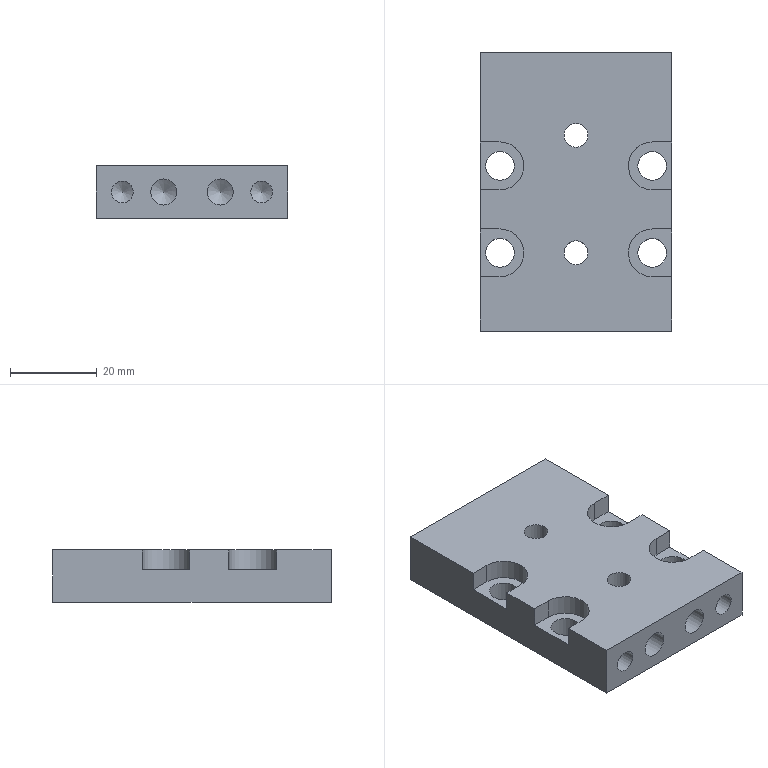Part | NX | features BREP 1 | 1 solid | 40 faces | box 44 x 64 x 12 mm | volume 28668 mm3 | plane 20 | cylinder 16 | cone 4 | commonest cylinder face diameters 6.6 x4 11 x4 5 x2 5.5 x2 6 x2 10 x2
STEP:
#1=CARTESIAN_POINT('',(-22.,-32.,0.));
#2=VERTEX_POINT('',#1);
#3=CARTESIAN_POINT('',(22.,-32.,0.));
#4=VERTEX_POINT('',#3);
#5=CARTESIAN_POINT('',(0.,-32.,0.));
#6=DIRECTION('',(1.,0.,0.));
#7=VECTOR('',#6,1000.);
#8=LINE('',#5,#7);
#9=EDGE_CURVE('',#2,#4,#8,.T.);
#10=ORIENTED_EDGE('',*,*,#9,.F.);
#11=CARTESIAN_POINT('',(-22.,32.,0.));
#12=VERTEX_POINT('',#11);
#13=CARTESIAN_POINT('',(-22.,0.,0.));
#14=DIRECTION('',(0.,-1.,0.));
#15=VECTOR('',#14,1000.);
#16=LINE('',#13,#15);
#17=EDGE_CURVE('',#12,#2,#16,.T.);
#18=ORIENTED_EDGE('',*,*,#17,.F.);
#19=CARTESIAN_POINT('',(22.,32.,0.));
#20=VERTEX_POINT('',#19);
#21=CARTESIAN_POINT('',(0.,32.,0.));
#22=DIRECTION('',(-1.,0.,0.));
#23=VECTOR('',#22,1000.);
#24=LINE('',#21,#23);
#25=EDGE_CURVE('',#20,#12,#24,.T.);
#26=ORIENTED_EDGE('',*,*,#25,.F.);
#27=CARTESIAN_POINT('',(22.,0.,0.));
#28=DIRECTION('',(0.,1.,0.));
#29=VECTOR('',#28,1000.);
#30=LINE('',#27,#29);
#31=EDGE_CURVE('',#4,#20,#30,.T.);
#32=ORIENTED_EDGE('',*,*,#31,.F.);
#33=EDGE_LOOP('',(#10,#18,#26,#32));
#34=FACE_BOUND('',#33,.T.);
#35=CARTESIAN_POINT('',(20.825,-14.,0.));
#36=VERTEX_POINT('',#35);
#37=CARTESIAN_POINT('',(17.525,-14.,0.));
#38=DIRECTION('',(0.,0.,-1.));
#39=DIRECTION('',(1.,0.,0.));
#40=AXIS2_PLACEMENT_3D('',#37,#38,#39);
#41=CIRCLE('',#40,3.3);
#42=EDGE_CURVE('',#36,#36,#41,.T.);
#43=ORIENTED_EDGE('',*,*,#42,.F.);
#44=EDGE_LOOP('',(#43));
#45=FACE_BOUND('',#44,.T.);
#46=CARTESIAN_POINT('',(20.825,6.,0.));
#47=VERTEX_POINT('',#46);
#48=CARTESIAN_POINT('',(17.525,6.,0.));
#49=DIRECTION('',(0.,0.,-1.));
#50=DIRECTION('',(1.,0.,0.));
#51=AXIS2_PLACEMENT_3D('',#48,#49,#50);
#52=CIRCLE('',#51,3.3);
#53=EDGE_CURVE('',#47,#47,#52,.T.);
#54=ORIENTED_EDGE('',*,*,#53,.F.);
#55=EDGE_LOOP('',(#54));
#56=FACE_BOUND('',#55,.T.);
#57=CARTESIAN_POINT('',(-14.175,-14.,0.));
#58=VERTEX_POINT('',#57);
#59=CARTESIAN_POINT('',(-17.475,-14.,0.));
#60=DIRECTION('',(0.,0.,-1.));
#61=DIRECTION('',(1.,0.,0.));
#62=AXIS2_PLACEMENT_3D('',#59,#60,#61);
#63=CIRCLE('',#62,3.3);
#64=EDGE_CURVE('',#58,#58,#63,.T.);
#65=ORIENTED_EDGE('',*,*,#64,.F.);
#66=EDGE_LOOP('',(#65));
#67=FACE_BOUND('',#66,.T.);
#68=CARTESIAN_POINT('',(-14.175,6.,0.));
#69=VERTEX_POINT('',#68);
#70=CARTESIAN_POINT('',(-17.475,6.,0.));
#71=DIRECTION('',(0.,0.,-1.));
#72=DIRECTION('',(1.,0.,0.));
#73=AXIS2_PLACEMENT_3D('',#70,#71,#72);
#74=CIRCLE('',#73,3.3);
#75=EDGE_CURVE('',#69,#69,#74,.T.);
#76=ORIENTED_EDGE('',*,*,#75,.F.);
#77=EDGE_LOOP('',(#76));
#78=FACE_BOUND('',#77,.T.);
#79=CARTESIAN_POINT('',(-5.,-14.,0.));
#80=VERTEX_POINT('',#79);
#81=CARTESIAN_POINT('',(0.,-14.,0.));
#82=DIRECTION('',(0.,0.,-1.));
#83=DIRECTION('',(-1.,0.,0.));
#84=AXIS2_PLACEMENT_3D('',#81,#82,#83);
#85=CIRCLE('',#84,5.);
#86=EDGE_CURVE('',#80,#80,#85,.T.);
#87=ORIENTED_EDGE('',*,*,#86,.F.);
#88=EDGE_LOOP('',(#87));
#89=FACE_BOUND('',#88,.T.);
#90=CARTESIAN_POINT('',(-5.,13.,0.));
#91=VERTEX_POINT('',#90);
#92=CARTESIAN_POINT('',(0.,13.,0.));
#93=DIRECTION('',(0.,0.,-1.));
#94=DIRECTION('',(-1.,0.,0.));
#95=AXIS2_PLACEMENT_3D('',#92,#93,#94);
#96=CIRCLE('',#95,5.);
#97=EDGE_CURVE('',#91,#91,#96,.T.);
#98=ORIENTED_EDGE('',*,*,#97,.F.);
#99=EDGE_LOOP('',(#98));
#100=FACE_BOUND('',#99,.T.);
#101=CARTESIAN_POINT('',(0.,0.,0.));
#102=DIRECTION('',(0.,0.,1.));
#103=DIRECTION('',(-1.,0.,0.));
#104=AXIS2_PLACEMENT_3D('',#101,#102,#103);
#105=PLANE('',#104);
#106=ADVANCED_FACE('',(#34,#45,#56,#67,#78,#89,#100),#105,.F.);
#107=CARTESIAN_POINT('',(22.,-19.5,12.));
#108=VERTEX_POINT('',#107);
#109=CARTESIAN_POINT('',(22.,-19.5,7.4));
#110=VERTEX_POINT('',#109);
#111=CARTESIAN_POINT('',(22.,-19.5,12.));
#112=DIRECTION('',(0.,0.,-1.));
#113=VECTOR('',#112,1000.);
#114=LINE('',#111,#113);
#115=EDGE_CURVE('',#108,#110,#114,.T.);
#116=ORIENTED_EDGE('',*,*,#115,.F.);
#117=CARTESIAN_POINT('',(22.,-32.,12.));
#118=VERTEX_POINT('',#117);
#119=CARTESIAN_POINT('',(22.,32.,12.));
#120=DIRECTION('',(0.,1.,0.));
#121=VECTOR('',#120,1000.);
#122=LINE('',#119,#121);
#123=EDGE_CURVE('',#118,#108,#122,.T.);
#124=ORIENTED_EDGE('',*,*,#123,.F.);
#125=CARTESIAN_POINT('',(22.,-32.,12.));
#126=DIRECTION('',(0.,0.,1.));
#127=VECTOR('',#126,1000.);
#128=LINE('',#125,#127);
#129=EDGE_CURVE('',#4,#118,#128,.T.);
#130=ORIENTED_EDGE('',*,*,#129,.F.);
#131=ORIENTED_EDGE('',*,*,#31,.T.);
#132=CARTESIAN_POINT('',(22.,32.,12.));
#133=VERTEX_POINT('',#132);
#134=CARTESIAN_POINT('',(22.,32.,12.));
#135=DIRECTION('',(0.,0.,-1.));
#136=VECTOR('',#135,1000.);
#137=LINE('',#134,#136);
#138=EDGE_CURVE('',#133,#20,#137,.T.);
#139=ORIENTED_EDGE('',*,*,#138,.F.);
#140=CARTESIAN_POINT('',(22.,11.5,12.));
#141=VERTEX_POINT('',#140);
#142=CARTESIAN_POINT('',(22.,32.,12.));
#143=DIRECTION('',(0.,1.,0.));
#144=VECTOR('',#143,1000.);
#145=LINE('',#142,#144);
#146=EDGE_CURVE('',#141,#133,#145,.T.);
#147=ORIENTED_EDGE('',*,*,#146,.F.);
#148=CARTESIAN_POINT('',(22.,11.5,7.4));
#149=VERTEX_POINT('',#148);
#150=CARTESIAN_POINT('',(22.,11.5,12.));
#151=DIRECTION('',(0.,0.,1.));
#152=VECTOR('',#151,1000.);
#153=LINE('',#150,#152);
#154=EDGE_CURVE('',#149,#141,#153,.T.);
#155=ORIENTED_EDGE('',*,*,#154,.F.);
#156=CARTESIAN_POINT('',(22.,0.5,7.4));
#157=VERTEX_POINT('',#156);
#158=CARTESIAN_POINT('',(22.,32.,7.4));
#159=DIRECTION('',(0.,1.,0.));
#160=VECTOR('',#159,1000.);
#161=LINE('',#158,#160);
#162=EDGE_CURVE('',#157,#149,#161,.T.);
#163=ORIENTED_EDGE('',*,*,#162,.F.);
#164=CARTESIAN_POINT('',(22.,0.5,12.));
#165=VERTEX_POINT('',#164);
#166=CARTESIAN_POINT('',(22.,0.5,12.));
#167=DIRECTION('',(0.,0.,-1.));
#168=VECTOR('',#167,1000.);
#169=LINE('',#166,#168);
#170=EDGE_CURVE('',#165,#157,#169,.T.);
#171=ORIENTED_EDGE('',*,*,#170,.F.);
#172=CARTESIAN_POINT('',(22.,-8.5,12.));
#173=VERTEX_POINT('',#172);
#174=CARTESIAN_POINT('',(22.,32.,12.));
#175=DIRECTION('',(0.,1.,0.));
#176=VECTOR('',#175,1000.);
#177=LINE('',#174,#176);
#178=EDGE_CURVE('',#173,#165,#177,.T.);
#179=ORIENTED_EDGE('',*,*,#178,.F.);
#180=CARTESIAN_POINT('',(22.,-8.5,7.4));
#181=VERTEX_POINT('',#180);
#182=CARTESIAN_POINT('',(22.,-8.5,12.));
#183=DIRECTION('',(0.,0.,1.));
#184=VECTOR('',#183,1000.);
#185=LINE('',#182,#184);
#186=EDGE_CURVE('',#181,#173,#185,.T.);
#187=ORIENTED_EDGE('',*,*,#186,.F.);
#188=CARTESIAN_POINT('',(22.,32.,7.4));
#189=DIRECTION('',(0.,1.,0.));
#190=VECTOR('',#189,1000.);
#191=LINE('',#188,#190);
#192=EDGE_CURVE('',#110,#181,#191,.T.);
#193=ORIENTED_EDGE('',*,*,#192,.F.);
#194=EDGE_LOOP('',(#116,#124,#130,#131,#139,#147,#155,#163,#171,#179,#187,#193));
#195=FACE_BOUND('',#194,.T.);
#196=CARTESIAN_POINT('',(22.,32.,12.));
#197=DIRECTION('',(-1.,0.,0.));
#198=DIRECTION('',(0.,1.,0.));
#199=AXIS2_PLACEMENT_3D('',#196,#197,#198);
#200=PLANE('',#199);
#201=ADVANCED_FACE('',(#195),#200,.F.);
#202=ORIENTED_EDGE('',*,*,#129,.T.);
#203=CARTESIAN_POINT('',(-22.,-32.,12.));
#204=VERTEX_POINT('',#203);
#205=CARTESIAN_POINT('',(-22.,-32.,12.));
#206=DIRECTION('',(1.,0.,0.));
#207=VECTOR('',#206,1000.);
#208=LINE('',#205,#207);
#209=EDGE_CURVE('',#204,#118,#208,.T.);
#210=ORIENTED_EDGE('',*,*,#209,.F.);
#211=CARTESIAN_POINT('',(-22.,-32.,12.));
#212=DIRECTION('',(0.,0.,1.));
#213=VECTOR('',#212,1000.);
#214=LINE('',#211,#213);
#215=EDGE_CURVE('',#2,#204,#214,.T.);
#216=ORIENTED_EDGE('',*,*,#215,.F.);
#217=ORIENTED_EDGE('',*,*,#9,.T.);
#218=EDGE_LOOP('',(#202,#210,#216,#217));
#219=FACE_BOUND('',#218,.T.);
#220=CARTESIAN_POINT('',(16.,-32.,3.5));
#221=VERTEX_POINT('',#220);
#222=CARTESIAN_POINT('',(16.,-32.,6.));
#223=DIRECTION('',(0.,-1.,0.));
#224=DIRECTION('',(0.,0.,-1.));
#225=AXIS2_PLACEMENT_3D('',#222,#223,#224);
#226=CIRCLE('',#225,2.5);
#227=EDGE_CURVE('',#221,#221,#226,.T.);
#228=ORIENTED_EDGE('',*,*,#227,.F.);
#229=EDGE_LOOP('',(#228));
#230=FACE_BOUND('',#229,.T.);
#231=CARTESIAN_POINT('',(-16.,-32.,3.5));
#232=VERTEX_POINT('',#231);
#233=CARTESIAN_POINT('',(-16.,-32.,6.));
#234=DIRECTION('',(0.,-1.,0.));
#235=DIRECTION('',(0.,0.,-1.));
#236=AXIS2_PLACEMENT_3D('',#233,#234,#235);
#237=CIRCLE('',#236,2.5);
#238=EDGE_CURVE('',#232,#232,#237,.T.);
#239=ORIENTED_EDGE('',*,*,#238,.F.);
#240=EDGE_LOOP('',(#239));
#241=FACE_BOUND('',#240,.T.);
#242=CARTESIAN_POINT('',(6.5,-32.,3.));
#243=VERTEX_POINT('',#242);
#244=CARTESIAN_POINT('',(6.5,-32.,6.));
#245=DIRECTION('',(0.,-1.,0.));
#246=DIRECTION('',(0.,0.,-1.));
#247=AXIS2_PLACEMENT_3D('',#244,#245,#246);
#248=CIRCLE('',#247,3.);
#249=EDGE_CURVE('',#243,#243,#248,.T.);
#250=ORIENTED_EDGE('',*,*,#249,.F.);
#251=EDGE_LOOP('',(#250));
#252=FACE_BOUND('',#251,.T.);
#253=CARTESIAN_POINT('',(-6.5,-32.,3.));
#254=VERTEX_POINT('',#253);
#255=CARTESIAN_POINT('',(-6.5,-32.,6.));
#256=DIRECTION('',(0.,-1.,0.));
#257=DIRECTION('',(0.,0.,-1.));
#258=AXIS2_PLACEMENT_3D('',#255,#256,#257);
#259=CIRCLE('',#258,3.);
#260=EDGE_CURVE('',#254,#254,#259,.T.);
#261=ORIENTED_EDGE('',*,*,#260,.F.);
#262=EDGE_LOOP('',(#261));
#263=FACE_BOUND('',#262,.T.);
#264=CARTESIAN_POINT('',(-22.,-32.,12.));
#265=DIRECTION('',(0.,1.,0.));
#266=DIRECTION('',(0.,0.,-1.));
#267=AXIS2_PLACEMENT_3D('',#264,#265,#266);
#268=PLANE('',#267);
#269=ADVANCED_FACE('',(#219,#230,#241,#252,#263),#268,.F.);
#270=CARTESIAN_POINT('',(-22.,-8.5,12.));
#271=VERTEX_POINT('',#270);
#272=CARTESIAN_POINT('',(-22.,-8.5,7.4));
#273=VERTEX_POINT('',#272);
#274=CARTESIAN_POINT('',(-22.,-8.5,12.));
#275=DIRECTION('',(0.,0.,-1.));
#276=VECTOR('',#275,1000.);
#277=LINE('',#274,#276);
#278=EDGE_CURVE('',#271,#273,#277,.T.);
#279=ORIENTED_EDGE('',*,*,#278,.F.);
#280=CARTESIAN_POINT('',(-22.,0.5,12.));
#281=VERTEX_POINT('',#280);
#282=CARTESIAN_POINT('',(-22.,32.,12.));
#283=DIRECTION('',(0.,-1.,0.));
#284=VECTOR('',#283,1000.);
#285=LINE('',#282,#284);
#286=EDGE_CURVE('',#281,#271,#285,.T.);
#287=ORIENTED_EDGE('',*,*,#286,.F.);
#288=CARTESIAN_POINT('',(-22.,0.5,7.4));
#289=VERTEX_POINT('',#288);
#290=CARTESIAN_POINT('',(-22.,0.5,12.));
#291=DIRECTION('',(0.,0.,1.));
#292=VECTOR('',#291,1000.);
#293=LINE('',#290,#292);
#294=EDGE_CURVE('',#289,#281,#293,.T.);
#295=ORIENTED_EDGE('',*,*,#294,.F.);
#296=CARTESIAN_POINT('',(-22.,11.5,7.4));
#297=VERTEX_POINT('',#296);
#298=CARTESIAN_POINT('',(-22.,32.,7.4));
#299=DIRECTION('',(0.,-1.,0.));
#300=VECTOR('',#299,1000.);
#301=LINE('',#298,#300);
#302=EDGE_CURVE('',#297,#289,#301,.T.);
#303=ORIENTED_EDGE('',*,*,#302,.F.);
#304=CARTESIAN_POINT('',(-22.,11.5,12.));
#305=VERTEX_POINT('',#304);
#306=CARTESIAN_POINT('',(-22.,11.5,12.));
#307=DIRECTION('',(0.,0.,-1.));
#308=VECTOR('',#307,1000.);
#309=LINE('',#306,#308);
#310=EDGE_CURVE('',#305,#297,#309,.T.);
#311=ORIENTED_EDGE('',*,*,#310,.F.);
#312=CARTESIAN_POINT('',(-22.,32.,12.));
#313=VERTEX_POINT('',#312);
#314=CARTESIAN_POINT('',(-22.,32.,12.));
#315=DIRECTION('',(0.,-1.,0.));
#316=VECTOR('',#315,1000.);
#317=LINE('',#314,#316);
#318=EDGE_CURVE('',#313,#305,#317,.T.);
#319=ORIENTED_EDGE('',*,*,#318,.F.);
#320=CARTESIAN_POINT('',(-22.,32.,12.));
#321=DIRECTION('',(0.,0.,1.));
#322=VECTOR('',#321,1000.);
#323=LINE('',#320,#322);
#324=EDGE_CURVE('',#12,#313,#323,.T.);
#325=ORIENTED_EDGE('',*,*,#324,.F.);
#326=ORIENTED_EDGE('',*,*,#17,.T.);
#327=ORIENTED_EDGE('',*,*,#215,.T.);
#328=CARTESIAN_POINT('',(-22.,-19.5,12.));
#329=VERTEX_POINT('',#328);
#330=CARTESIAN_POINT('',(-22.,32.,12.));
#331=DIRECTION('',(0.,-1.,0.));
#332=VECTOR('',#331,1000.);
#333=LINE('',#330,#332);
#334=EDGE_CURVE('',#329,#204,#333,.T.);
#335=ORIENTED_EDGE('',*,*,#334,.F.);
#336=CARTESIAN_POINT('',(-22.,-19.5,7.4));
#337=VERTEX_POINT('',#336);
#338=CARTESIAN_POINT('',(-22.,-19.5,12.));
#339=DIRECTION('',(0.,0.,1.));
#340=VECTOR('',#339,1000.);
#341=LINE('',#338,#340);
#342=EDGE_CURVE('',#337,#329,#341,.T.);
#343=ORIENTED_EDGE('',*,*,#342,.F.);
#344=CARTESIAN_POINT('',(-22.,32.,7.4));
#345=DIRECTION('',(0.,-1.,0.));
#346=VECTOR('',#345,1000.);
#347=LINE('',#344,#346);
#348=EDGE_CURVE('',#273,#337,#347,.T.);
#349=ORIENTED_EDGE('',*,*,#348,.F.);
#350=EDGE_LOOP('',(#279,#287,#295,#303,#311,#319,#325,#326,#327,#335,#343,#349));
#351=FACE_BOUND('',#350,.T.);
#352=CARTESIAN_POINT('',(-22.,32.,12.));
#353=DIRECTION('',(1.,0.,0.));
#354=DIRECTION('',(0.,-1.,0.));
#355=AXIS2_PLACEMENT_3D('',#352,#353,#354);
#356=PLANE('',#355);
#357=ADVANCED_FACE('',(#351),#356,.F.);
#358=ORIENTED_EDGE('',*,*,#324,.T.);
#359=CARTESIAN_POINT('',(-22.,32.,12.));
#360=DIRECTION('',(-1.,0.,0.));
#361=VECTOR('',#360,1000.);
#362=LINE('',#359,#361);
#363=EDGE_CURVE('',#133,#313,#362,.T.);
#364=ORIENTED_EDGE('',*,*,#363,.F.);
#365=ORIENTED_EDGE('',*,*,#138,.T.);
#366=ORIENTED_EDGE('',*,*,#25,.T.);
#367=EDGE_LOOP('',(#358,#364,#365,#366));
#368=FACE_BOUND('',#367,.T.);
#369=CARTESIAN_POINT('',(-22.,32.,12.));
#370=DIRECTION('',(0.,-1.,0.));
#371=DIRECTION('',(0.,0.,1.));
#372=AXIS2_PLACEMENT_3D('',#369,#370,#371);
#373=PLANE('',#372);
#374=ADVANCED_FACE('',(#368),#373,.F.);
#375=ORIENTED_EDGE('',*,*,#42,.T.);
#376=EDGE_LOOP('',(#375));
#377=FACE_BOUND('',#376,.T.);
#378=CARTESIAN_POINT('',(20.825,-14.,7.4));
#379=VERTEX_POINT('',#378);
#380=CARTESIAN_POINT('',(17.525,-14.,7.4));
#381=DIRECTION('',(0.,0.,-1.));
#382=DIRECTION('',(1.,0.,0.));
#383=AXIS2_PLACEMENT_3D('',#380,#381,#382);
#384=CIRCLE('',#383,3.3);
#385=EDGE_CURVE('',#379,#379,#384,.T.);
#386=ORIENTED_EDGE('',*,*,#385,.F.);
#387=EDGE_LOOP('',(#386));
#388=FACE_BOUND('',#387,.T.);
#389=CARTESIAN_POINT('',(17.525,-14.,12.));
#390=DIRECTION('',(0.,0.,1.));
#391=DIRECTION('',(-1.,0.,0.));
#392=AXIS2_PLACEMENT_3D('',#389,#390,#391);
#393=CYLINDRICAL_SURFACE('',#392,3.3);
#394=ADVANCED_FACE('',(#377,#388),#393,.F.);
#395=ORIENTED_EDGE('',*,*,#53,.T.);
#396=EDGE_LOOP('',(#395));
#397=FACE_BOUND('',#396,.T.);
#398=CARTESIAN_POINT('',(20.825,6.,7.4));
#399=VERTEX_POINT('',#398);
#400=CARTESIAN_POINT('',(17.525,6.,7.4));
#401=DIRECTION('',(0.,0.,-1.));
#402=DIRECTION('',(1.,0.,0.));
#403=AXIS2_PLACEMENT_3D('',#400,#401,#402);
#404=CIRCLE('',#403,3.3);
#405=EDGE_CURVE('',#399,#399,#404,.T.);
#406=ORIENTED_EDGE('',*,*,#405,.F.);
#407=EDGE_LOOP('',(#406));
#408=FACE_BOUND('',#407,.T.);
#409=CARTESIAN_POINT('',(17.525,6.,12.));
#410=DIRECTION('',(0.,0.,1.));
#411=DIRECTION('',(-1.,0.,0.));
#412=AXIS2_PLACEMENT_3D('',#409,#410,#411);
#413=CYLINDRICAL_SURFACE('',#412,3.3);
#414=ADVANCED_FACE('',(#397,#408),#413,.F.);
#415=ORIENTED_EDGE('',*,*,#64,.T.);
#416=EDGE_LOOP('',(#415));
#417=FACE_BOUND('',#416,.T.);
#418=CARTESIAN_POINT('',(-14.175,-14.,7.4));
#419=VERTEX_POINT('',#418);
#420=CARTESIAN_POINT('',(-17.475,-14.,7.4));
#421=DIRECTION('',(0.,0.,-1.));
#422=DIRECTION('',(1.,0.,0.));
#423=AXIS2_PLACEMENT_3D('',#420,#421,#422);
#424=CIRCLE('',#423,3.3);
#425=EDGE_CURVE('',#419,#419,#424,.T.);
#426=ORIENTED_EDGE('',*,*,#425,.F.);
#427=EDGE_LOOP('',(#426));
#428=FACE_BOUND('',#427,.T.);
#429=CARTESIAN_POINT('',(-17.475,-14.,12.));
#430=DIRECTION('',(0.,0.,1.));
#431=DIRECTION('',(-1.,0.,0.));
#432=AXIS2_PLACEMENT_3D('',#429,#430,#431);
#433=CYLINDRICAL_SURFACE('',#432,3.3);
#434=ADVANCED_FACE('',(#417,#428),#433,.F.);
#435=ORIENTED_EDGE('',*,*,#75,.T.);
#436=EDGE_LOOP('',(#435));
#437=FACE_BOUND('',#436,.T.);
#438=CARTESIAN_POINT('',(-14.175,6.,7.4));
#439=VERTEX_POINT('',#438);
#440=CARTESIAN_POINT('',(-17.475,6.,7.4));
#441=DIRECTION('',(0.,0.,-1.));
#442=DIRECTION('',(1.,0.,0.));
#443=AXIS2_PLACEMENT_3D('',#440,#441,#442);
#444=CIRCLE('',#443,3.3);
#445=EDGE_CURVE('',#439,#439,#444,.T.);
#446=ORIENTED_EDGE('',*,*,#445,.F.);
#447=EDGE_LOOP('',(#446));
#448=FACE_BOUND('',#447,.T.);
#449=CARTESIAN_POINT('',(-17.475,6.,12.));
#450=DIRECTION('',(0.,0.,1.));
#451=DIRECTION('',(-1.,0.,0.));
#452=AXIS2_PLACEMENT_3D('',#449,#450,#451);
#453=CYLINDRICAL_SURFACE('',#452,3.3);
#454=ADVANCED_FACE('',(#437,#448),#453,.F.);
#455=CARTESIAN_POINT('',(-5.,-14.,5.4));
#456=VERTEX_POINT('',#455);
#457=CARTESIAN_POINT('',(0.,-14.,5.4));
#458=DIRECTION('',(0.,0.,-1.));
#459=DIRECTION('',(-1.,0.,0.));
#460=AXIS2_PLACEMENT_3D('',#457,#458,#459);
#461=CIRCLE('',#460,5.);
#462=EDGE_CURVE('',#456,#456,#461,.T.);
#463=ORIENTED_EDGE('',*,*,#462,.F.);
#464=EDGE_LOOP('',(#463));
#465=FACE_BOUND('',#464,.T.);
#466=ORIENTED_EDGE('',*,*,#86,.T.);
#467=EDGE_LOOP('',(#466));
#468=FACE_BOUND('',#467,.T.);
#469=CARTESIAN_POINT('',(0.,-14.,0.));
#470=DIRECTION('',(0.,0.,-1.));
#471=DIRECTION('',(1.,0.,0.));
#472=AXIS2_PLACEMENT_3D('',#469,#470,#471);
#473=CYLINDRICAL_SURFACE('',#472,5.);
#474=ADVANCED_FACE('',(#465,#468),#473,.F.);
#475=CARTESIAN_POINT('',(-5.,13.,5.4));
#476=VERTEX_POINT('',#475);
#477=CARTESIAN_POINT('',(0.,13.,5.4));
#478=DIRECTION('',(0.,0.,-1.));
#479=DIRECTION('',(-1.,0.,0.));
#480=AXIS2_PLACEMENT_3D('',#477,#478,#479);
#481=CIRCLE('',#480,5.);
#482=EDGE_CURVE('',#476,#476,#481,.T.);
#483=ORIENTED_EDGE('',*,*,#482,.F.);
#484=EDGE_LOOP('',(#483));
#485=FACE_BOUND('',#484,.T.);
#486=ORIENTED_EDGE('',*,*,#97,.T.);
#487=EDGE_LOOP('',(#486));
#488=FACE_BOUND('',#487,.T.);
#489=CARTESIAN_POINT('',(0.,13.,0.));
#490=DIRECTION('',(0.,0.,-1.));
#491=DIRECTION('',(1.,0.,0.));
#492=AXIS2_PLACEMENT_3D('',#489,#490,#491);
#493=CYLINDRICAL_SURFACE('',#492,5.);
#494=ADVANCED_FACE('',(#485,#488),#493,.F.);
#495=CARTESIAN_POINT('',(17.525,-19.5,7.4));
#496=VERTEX_POINT('',#495);
#497=CARTESIAN_POINT('',(20.825,-19.5,7.4));
#498=DIRECTION('',(-1.,0.,0.));
#499=VECTOR('',#498,1000.);
#500=LINE('',#497,#499);
#501=EDGE_CURVE('',#110,#496,#500,.T.);
#502=ORIENTED_EDGE('',*,*,#501,.F.);
#503=ORIENTED_EDGE('',*,*,#192,.T.);
#504=CARTESIAN_POINT('',(17.525,-8.5,7.4));
#505=VERTEX_POINT('',#504);
#506=CARTESIAN_POINT('',(20.825,-8.5,7.4));
#507=DIRECTION('',(1.,0.,0.));
#508=VECTOR('',#507,1000.);
#509=LINE('',#506,#508);
#510=EDGE_CURVE('',#505,#181,#509,.T.);
#511=ORIENTED_EDGE('',*,*,#510,.F.);
#512=CARTESIAN_POINT('',(17.525,-14.,7.4));
#513=DIRECTION('',(0.,0.,-1.));
#514=DIRECTION('',(1.,0.,0.));
#515=AXIS2_PLACEMENT_3D('',#512,#513,#514);
#516=CIRCLE('',#515,5.5);
#517=EDGE_CURVE('',#496,#505,#516,.T.);
#518=ORIENTED_EDGE('',*,*,#517,.F.);
#519=EDGE_LOOP('',(#502,#503,#511,#518));
#520=FACE_BOUND('',#519,.T.);
#521=ORIENTED_EDGE('',*,*,#385,.T.);
#522=EDGE_LOOP('',(#521));
#523=FACE_BOUND('',#522,.T.);
#524=CARTESIAN_POINT('',(20.825,-14.,7.4));
#525=DIRECTION('',(0.,0.,-1.));
#526=DIRECTION('',(1.,0.,0.));
#527=AXIS2_PLACEMENT_3D('',#524,#525,#526);
#528=PLANE('',#527);
#529=ADVANCED_FACE('',(#520,#523),#528,.F.);
#530=CARTESIAN_POINT('',(17.525,-19.5,12.));
#531=VERTEX_POINT('',#530);
#532=CARTESIAN_POINT('',(22.,-19.5,12.));
#533=DIRECTION('',(-1.,0.,0.));
#534=VECTOR('',#533,1000.);
#535=LINE('',#532,#534);
#536=EDGE_CURVE('',#108,#531,#535,.T.);
#537=ORIENTED_EDGE('',*,*,#536,.F.);
#538=ORIENTED_EDGE('',*,*,#115,.T.);
#539=ORIENTED_EDGE('',*,*,#501,.T.);
#540=CARTESIAN_POINT('',(17.525,-19.5,-4.494));
#541=DIRECTION('',(0.,0.,-1.));
#542=VECTOR('',#541,1000.);
#543=LINE('',#540,#542);
#544=EDGE_CURVE('',#531,#496,#543,.T.);
#545=ORIENTED_EDGE('',*,*,#544,.F.);
#546=EDGE_LOOP('',(#537,#538,#539,#545));
#547=FACE_BOUND('',#546,.T.);
#548=CARTESIAN_POINT('',(22.,-19.5,-4.494));
#549=DIRECTION('',(0.,-1.,0.));
#550=DIRECTION('',(-1.,0.,0.));
#551=AXIS2_PLACEMENT_3D('',#548,#549,#550);
#552=PLANE('',#551);
#553=ADVANCED_FACE('',(#547),#552,.F.);
#554=ORIENTED_EDGE('',*,*,#209,.T.);
#555=ORIENTED_EDGE('',*,*,#123,.T.);
#556=ORIENTED_EDGE('',*,*,#536,.T.);
#557=CARTESIAN_POINT('',(17.525,-8.5,12.));
#558=VERTEX_POINT('',#557);
#559=CARTESIAN_POINT('',(17.525,-14.,12.));
#560=DIRECTION('',(0.,0.,-1.));
#561=DIRECTION('',(1.,0.,0.));
#562=AXIS2_PLACEMENT_3D('',#559,#560,#561);
#563=CIRCLE('',#562,5.5);
#564=EDGE_CURVE('',#531,#558,#563,.T.);
#565=ORIENTED_EDGE('',*,*,#564,.T.);
#566=CARTESIAN_POINT('',(0.,-8.5,12.));
#567=DIRECTION('',(1.,0.,0.));
#568=VECTOR('',#567,1000.);
#569=LINE('',#566,#568);
#570=EDGE_CURVE('',#558,#173,#569,.T.);
#571=ORIENTED_EDGE('',*,*,#570,.T.);
#572=ORIENTED_EDGE('',*,*,#178,.T.);
#573=CARTESIAN_POINT('',(17.525,0.5,12.));
#574=VERTEX_POINT('',#573);
#575=CARTESIAN_POINT('',(0.,0.5,12.));
#576=DIRECTION('',(-1.,0.,0.));
#577=VECTOR('',#576,1000.);
#578=LINE('',#575,#577);
#579=EDGE_CURVE('',#165,#574,#578,.T.);
#580=ORIENTED_EDGE('',*,*,#579,.T.);
#581=CARTESIAN_POINT('',(17.525,11.5,12.));
#582=VERTEX_POINT('',#581);
#583=CARTESIAN_POINT('',(17.525,6.,12.));
#584=DIRECTION('',(0.,0.,-1.));
#585=DIRECTION('',(1.,0.,0.));
#586=AXIS2_PLACEMENT_3D('',#583,#584,#585);
#587=CIRCLE('',#586,5.5);
#588=EDGE_CURVE('',#574,#582,#587,.T.);
#589=ORIENTED_EDGE('',*,*,#588,.T.);
#590=CARTESIAN_POINT('',(0.,11.5,12.));
#591=DIRECTION('',(1.,0.,0.));
#592=VECTOR('',#591,1000.);
#593=LINE('',#590,#592);
#594=EDGE_CURVE('',#582,#141,#593,.T.);
#595=ORIENTED_EDGE('',*,*,#594,.T.);
#596=ORIENTED_EDGE('',*,*,#146,.T.);
#597=ORIENTED_EDGE('',*,*,#363,.T.);
#598=ORIENTED_EDGE('',*,*,#318,.T.);
#599=CARTESIAN_POINT('',(-17.475,11.5,12.));
#600=VERTEX_POINT('',#599);
#601=CARTESIAN_POINT('',(0.,11.5,12.));
#602=DIRECTION('',(1.,0.,0.));
#603=VECTOR('',#602,1000.);
#604=LINE('',#601,#603);
#605=EDGE_CURVE('',#305,#600,#604,.T.);
#606=ORIENTED_EDGE('',*,*,#605,.T.);
#607=CARTESIAN_POINT('',(-17.475,0.5,12.));
#608=VERTEX_POINT('',#607);
#609=CARTESIAN_POINT('',(-17.475,6.,12.));
#610=DIRECTION('',(0.,0.,-1.));
#611=DIRECTION('',(1.,0.,0.));
#612=AXIS2_PLACEMENT_3D('',#609,#610,#611);
#613=CIRCLE('',#612,5.5);
#614=EDGE_CURVE('',#600,#608,#613,.T.);
#615=ORIENTED_EDGE('',*,*,#614,.T.);
#616=CARTESIAN_POINT('',(0.,0.5,12.));
#617=DIRECTION('',(-1.,0.,0.));
#618=VECTOR('',#617,1000.);
#619=LINE('',#616,#618);
#620=EDGE_CURVE('',#608,#281,#619,.T.);
#621=ORIENTED_EDGE('',*,*,#620,.T.);
#622=ORIENTED_EDGE('',*,*,#286,.T.);
#623=CARTESIAN_POINT('',(-17.475,-8.5,12.));
#624=VERTEX_POINT('',#623);
#625=CARTESIAN_POINT('',(0.,-8.5,12.));
#626=DIRECTION('',(1.,0.,0.));
#627=VECTOR('',#626,1000.);
#628=LINE('',#625,#627);
#629=EDGE_CURVE('',#271,#624,#628,.T.);
#630=ORIENTED_EDGE('',*,*,#629,.T.);
#631=CARTESIAN_POINT('',(-17.475,-19.5,12.));
#632=VERTEX_POINT('',#631);
#633=CARTESIAN_POINT('',(-17.475,-14.,12.));
#634=DIRECTION('',(0.,0.,-1.));
#635=DIRECTION('',(1.,0.,0.));
#636=AXIS2_PLACEMENT_3D('',#633,#634,#635);
#637=CIRCLE('',#636,5.5);
#638=EDGE_CURVE('',#624,#632,#637,.T.);
#639=ORIENTED_EDGE('',*,*,#638,.T.);
#640=CARTESIAN_POINT('',(0.,-19.5,12.));
#641=DIRECTION('',(-1.,0.,0.));
#642=VECTOR('',#641,1000.);
#643=LINE('',#640,#642);
#644=EDGE_CURVE('',#632,#329,#643,.T.);
#645=ORIENTED_EDGE('',*,*,#644,.T.);
#646=ORIENTED_EDGE('',*,*,#334,.T.);
#647=EDGE_LOOP('',(#554,#555,#556,#565,#571,#572,#580,#589,#595,#596,#597,#598,#606,#615,#621,#622,#630,#639,#645,#646));
#648=FACE_BOUND('',#647,.T.);
#649=CARTESIAN_POINT('',(-2.75,-14.,12.));
#650=VERTEX_POINT('',#649);
#651=CARTESIAN_POINT('',(0.,-14.,12.));
#652=DIRECTION('',(0.,0.,-1.));
#653=DIRECTION('',(-1.,0.,0.));
#654=AXIS2_PLACEMENT_3D('',#651,#652,#653);
#655=CIRCLE('',#654,2.75);
#656=EDGE_CURVE('',#650,#650,#655,.T.);
#657=ORIENTED_EDGE('',*,*,#656,.T.);
#658=EDGE_LOOP('',(#657));
#659=FACE_BOUND('',#658,.T.);
#660=CARTESIAN_POINT('',(-2.75,13.,12.));
#661=VERTEX_POINT('',#660);
#662=CARTESIAN_POINT('',(0.,13.,12.));
#663=DIRECTION('',(0.,0.,-1.));
#664=DIRECTION('',(-1.,0.,0.));
#665=AXIS2_PLACEMENT_3D('',#662,#663,#664);
#666=CIRCLE('',#665,2.75);
#667=EDGE_CURVE('',#661,#661,#666,.T.);
#668=ORIENTED_EDGE('',*,*,#667,.T.);
#669=EDGE_LOOP('',(#668));
#670=FACE_BOUND('',#669,.T.);
#671=CARTESIAN_POINT('',(0.,0.,12.));
#672=DIRECTION('',(0.,0.,1.));
#673=DIRECTION('',(-1.,0.,0.));
#674=AXIS2_PLACEMENT_3D('',#671,#672,#673);
#675=PLANE('',#674);
#676=ADVANCED_FACE('',(#648,#659,#670),#675,.T.);
#677=ORIENTED_EDGE('',*,*,#594,.F.);
#678=CARTESIAN_POINT('',(17.525,11.5,7.4));
#679=VERTEX_POINT('',#678);
#680=CARTESIAN_POINT('',(17.525,11.5,-4.494));
#681=DIRECTION('',(0.,0.,1.));
#682=VECTOR('',#681,1000.);
#683=LINE('',#680,#682);
#684=EDGE_CURVE('',#679,#582,#683,.T.);
#685=ORIENTED_EDGE('',*,*,#684,.F.);
#686=CARTESIAN_POINT('',(17.525,11.5,7.4));
#687=DIRECTION('',(-1.,0.,0.));
#688=VECTOR('',#687,1000.);
#689=LINE('',#686,#688);
#690=EDGE_CURVE('',#149,#679,#689,.T.);
#691=ORIENTED_EDGE('',*,*,#690,.F.);
#692=ORIENTED_EDGE('',*,*,#154,.T.);
#693=EDGE_LOOP('',(#677,#685,#691,#692));
#694=FACE_BOUND('',#693,.T.);
#695=CARTESIAN_POINT('',(17.525,11.5,-4.494));
#696=DIRECTION('',(0.,1.,0.));
#697=DIRECTION('',(0.,0.,-1.));
#698=AXIS2_PLACEMENT_3D('',#695,#696,#697);
#699=PLANE('',#698);
#700=ADVANCED_FACE('',(#694),#699,.F.);
#701=CARTESIAN_POINT('',(17.525,0.5,7.4));
#702=VERTEX_POINT('',#701);
#703=CARTESIAN_POINT('',(20.825,0.5,7.4));
#704=DIRECTION('',(-1.,0.,0.));
#705=VECTOR('',#704,1000.);
#706=LINE('',#703,#705);
#707=EDGE_CURVE('',#157,#702,#706,.T.);
#708=ORIENTED_EDGE('',*,*,#707,.F.);
#709=ORIENTED_EDGE('',*,*,#162,.T.);
#710=ORIENTED_EDGE('',*,*,#690,.T.);
#711=CARTESIAN_POINT('',(17.525,6.,7.4));
#712=DIRECTION('',(0.,0.,-1.));
#713=DIRECTION('',(1.,0.,0.));
#714=AXIS2_PLACEMENT_3D('',#711,#712,#713);
#715=CIRCLE('',#714,5.5);
#716=EDGE_CURVE('',#702,#679,#715,.T.);
#717=ORIENTED_EDGE('',*,*,#716,.F.);
#718=EDGE_LOOP('',(#708,#709,#710,#717));
#719=FACE_BOUND('',#718,.T.);
#720=ORIENTED_EDGE('',*,*,#405,.T.);
#721=EDGE_LOOP('',(#720));
#722=FACE_BOUND('',#721,.T.);
#723=CARTESIAN_POINT('',(20.825,6.,7.4));
#724=DIRECTION('',(0.,0.,-1.));
#725=DIRECTION('',(1.,0.,0.));
#726=AXIS2_PLACEMENT_3D('',#723,#724,#725);
#727=PLANE('',#726);
#728=ADVANCED_FACE('',(#719,#722),#727,.F.);
#729=ORIENTED_EDGE('',*,*,#579,.F.);
#730=ORIENTED_EDGE('',*,*,#170,.T.);
#731=ORIENTED_EDGE('',*,*,#707,.T.);
#732=CARTESIAN_POINT('',(17.525,0.5,-4.494));
#733=DIRECTION('',(0.,0.,-1.));
#734=VECTOR('',#733,1000.);
#735=LINE('',#732,#734);
#736=EDGE_CURVE('',#574,#702,#735,.T.);
#737=ORIENTED_EDGE('',*,*,#736,.F.);
#738=EDGE_LOOP('',(#729,#730,#731,#737));
#739=FACE_BOUND('',#738,.T.);
#740=CARTESIAN_POINT('',(22.,0.5,-4.494));
#741=DIRECTION('',(0.,-1.,0.));
#742=DIRECTION('',(-1.,0.,0.));
#743=AXIS2_PLACEMENT_3D('',#740,#741,#742);
#744=PLANE('',#743);
#745=ADVANCED_FACE('',(#739),#744,.F.);
#746=ORIENTED_EDGE('',*,*,#570,.F.);
#747=CARTESIAN_POINT('',(17.525,-8.5,-4.494));
#748=DIRECTION('',(0.,0.,1.));
#749=VECTOR('',#748,1000.);
#750=LINE('',#747,#749);
#751=EDGE_CURVE('',#505,#558,#750,.T.);
#752=ORIENTED_EDGE('',*,*,#751,.F.);
#753=ORIENTED_EDGE('',*,*,#510,.T.);
#754=ORIENTED_EDGE('',*,*,#186,.T.);
#755=EDGE_LOOP('',(#746,#752,#753,#754));
#756=FACE_BOUND('',#755,.T.);
#757=CARTESIAN_POINT('',(17.525,-8.5,-4.494));
#758=DIRECTION('',(0.,1.,0.));
#759=DIRECTION('',(1.,0.,0.));
#760=AXIS2_PLACEMENT_3D('',#757,#758,#759);
#761=PLANE('',#760);
#762=ADVANCED_FACE('',(#756),#761,.F.);
#763=CARTESIAN_POINT('',(16.,-21.,3.5));
#764=VERTEX_POINT('',#763);
#765=CARTESIAN_POINT('',(16.,-21.,6.));
#766=DIRECTION('',(0.,-1.,0.));
#767=DIRECTION('',(0.,0.,-1.));
#768=AXIS2_PLACEMENT_3D('',#765,#766,#767);
#769=CIRCLE('',#768,2.5);
#770=EDGE_CURVE('',#764,#764,#769,.T.);
#771=ORIENTED_EDGE('',*,*,#770,.F.);
#772=EDGE_LOOP('',(#771));
#773=FACE_BOUND('',#772,.T.);
#774=ORIENTED_EDGE('',*,*,#227,.T.);
#775=EDGE_LOOP('',(#774));
#776=FACE_BOUND('',#775,.T.);
#777=CARTESIAN_POINT('',(16.,-32.,6.));
#778=DIRECTION('',(0.,-1.,0.));
#779=DIRECTION('',(0.,0.,1.));
#780=AXIS2_PLACEMENT_3D('',#777,#778,#779);
#781=CYLINDRICAL_SURFACE('',#780,2.5);
#782=ADVANCED_FACE('',(#773,#776),#781,.F.);
#783=CARTESIAN_POINT('',(-16.,-21.,3.5));
#784=VERTEX_POINT('',#783);
#785=CARTESIAN_POINT('',(-16.,-21.,6.));
#786=DIRECTION('',(0.,-1.,0.));
#787=DIRECTION('',(0.,0.,-1.));
#788=AXIS2_PLACEMENT_3D('',#785,#786,#787);
#789=CIRCLE('',#788,2.5);
#790=EDGE_CURVE('',#784,#784,#789,.T.);
#791=ORIENTED_EDGE('',*,*,#790,.F.);
#792=EDGE_LOOP('',(#791));
#793=FACE_BOUND('',#792,.T.);
#794=ORIENTED_EDGE('',*,*,#238,.T.);
#795=EDGE_LOOP('',(#794));
#796=FACE_BOUND('',#795,.T.);
#797=CARTESIAN_POINT('',(-16.,-32.,6.));
#798=DIRECTION('',(0.,-1.,0.));
#799=DIRECTION('',(0.,0.,1.));
#800=AXIS2_PLACEMENT_3D('',#797,#798,#799);
#801=CYLINDRICAL_SURFACE('',#800,2.5);
#802=ADVANCED_FACE('',(#793,#796),#801,.F.);
#803=CARTESIAN_POINT('',(6.5,-20.,3.));
#804=VERTEX_POINT('',#803);
#805=CARTESIAN_POINT('',(6.5,-20.,6.));
#806=DIRECTION('',(0.,-1.,0.));
#807=DIRECTION('',(0.,0.,-1.));
#808=AXIS2_PLACEMENT_3D('',#805,#806,#807);
#809=CIRCLE('',#808,3.);
#810=EDGE_CURVE('',#804,#804,#809,.T.);
#811=ORIENTED_EDGE('',*,*,#810,.F.);
#812=EDGE_LOOP('',(#811));
#813=FACE_BOUND('',#812,.T.);
#814=ORIENTED_EDGE('',*,*,#249,.T.);
#815=EDGE_LOOP('',(#814));
#816=FACE_BOUND('',#815,.T.);
#817=CARTESIAN_POINT('',(6.5,-32.,6.));
#818=DIRECTION('',(0.,-1.,0.));
#819=DIRECTION('',(0.,0.,1.));
#820=AXIS2_PLACEMENT_3D('',#817,#818,#819);
#821=CYLINDRICAL_SURFACE('',#820,3.);
#822=ADVANCED_FACE('',(#813,#816),#821,.F.);
#823=CARTESIAN_POINT('',(-6.5,-20.,3.));
#824=VERTEX_POINT('',#823);
#825=CARTESIAN_POINT('',(-6.5,-20.,6.));
#826=DIRECTION('',(0.,-1.,0.));
#827=DIRECTION('',(0.,0.,-1.));
#828=AXIS2_PLACEMENT_3D('',#825,#826,#827);
#829=CIRCLE('',#828,3.);
#830=EDGE_CURVE('',#824,#824,#829,.T.);
#831=ORIENTED_EDGE('',*,*,#830,.F.);
#832=EDGE_LOOP('',(#831));
#833=FACE_BOUND('',#832,.T.);
#834=ORIENTED_EDGE('',*,*,#260,.T.);
#835=EDGE_LOOP('',(#834));
#836=FACE_BOUND('',#835,.T.);
#837=CARTESIAN_POINT('',(-6.5,-32.,6.));
#838=DIRECTION('',(0.,-1.,0.));
#839=DIRECTION('',(0.,0.,1.));
#840=AXIS2_PLACEMENT_3D('',#837,#838,#839);
#841=CYLINDRICAL_SURFACE('',#840,3.);
#842=ADVANCED_FACE('',(#833,#836),#841,.F.);
#843=CARTESIAN_POINT('',(-17.475,-8.5,7.4));
#844=VERTEX_POINT('',#843);
#845=CARTESIAN_POINT('',(-17.475,-19.5,7.4));
#846=VERTEX_POINT('',#845);
#847=CARTESIAN_POINT('',(-17.475,-14.,7.4));
#848=DIRECTION('',(0.,0.,-1.));
#849=DIRECTION('',(1.,0.,0.));
#850=AXIS2_PLACEMENT_3D('',#847,#848,#849);
#851=CIRCLE('',#850,5.5);
#852=EDGE_CURVE('',#844,#846,#851,.T.);
#853=ORIENTED_EDGE('',*,*,#852,.F.);
#854=CARTESIAN_POINT('',(-14.175,-8.5,7.4));
#855=DIRECTION('',(1.,0.,0.));
#856=VECTOR('',#855,1000.);
#857=LINE('',#854,#856);
#858=EDGE_CURVE('',#273,#844,#857,.T.);
#859=ORIENTED_EDGE('',*,*,#858,.F.);
#860=ORIENTED_EDGE('',*,*,#348,.T.);
#861=CARTESIAN_POINT('',(-14.175,-19.5,7.4));
#862=DIRECTION('',(-1.,0.,0.));
#863=VECTOR('',#862,1000.);
#864=LINE('',#861,#863);
#865=EDGE_CURVE('',#846,#337,#864,.T.);
#866=ORIENTED_EDGE('',*,*,#865,.F.);
#867=EDGE_LOOP('',(#853,#859,#860,#866));
#868=FACE_BOUND('',#867,.T.);
#869=ORIENTED_EDGE('',*,*,#425,.T.);
#870=EDGE_LOOP('',(#869));
#871=FACE_BOUND('',#870,.T.);
#872=CARTESIAN_POINT('',(-14.175,-14.,7.4));
#873=DIRECTION('',(0.,0.,-1.));
#874=DIRECTION('',(1.,0.,0.));
#875=AXIS2_PLACEMENT_3D('',#872,#873,#874);
#876=PLANE('',#875);
#877=ADVANCED_FACE('',(#868,#871),#876,.F.);
#878=ORIENTED_EDGE('',*,*,#629,.F.);
#879=ORIENTED_EDGE('',*,*,#278,.T.);
#880=ORIENTED_EDGE('',*,*,#858,.T.);
#881=CARTESIAN_POINT('',(-17.475,-8.5,-4.494));
#882=DIRECTION('',(0.,0.,-1.));
#883=VECTOR('',#882,1000.);
#884=LINE('',#881,#883);
#885=EDGE_CURVE('',#624,#844,#884,.T.);
#886=ORIENTED_EDGE('',*,*,#885,.F.);
#887=EDGE_LOOP('',(#878,#879,#880,#886));
#888=FACE_BOUND('',#887,.T.);
#889=CARTESIAN_POINT('',(-17.475,-8.5,-4.494));
#890=DIRECTION('',(0.,1.,0.));
#891=DIRECTION('',(1.,0.,0.));
#892=AXIS2_PLACEMENT_3D('',#889,#890,#891);
#893=PLANE('',#892);
#894=ADVANCED_FACE('',(#888),#893,.F.);
#895=ORIENTED_EDGE('',*,*,#620,.F.);
#896=CARTESIAN_POINT('',(-17.475,0.5,7.4));
#897=VERTEX_POINT('',#896);
#898=CARTESIAN_POINT('',(-17.475,0.5,-4.494));
#899=DIRECTION('',(0.,0.,1.));
#900=VECTOR('',#899,1000.);
#901=LINE('',#898,#900);
#902=EDGE_CURVE('',#897,#608,#901,.T.);
#903=ORIENTED_EDGE('',*,*,#902,.F.);
#904=CARTESIAN_POINT('',(-22.,0.5,7.4));
#905=DIRECTION('',(1.,0.,0.));
#906=VECTOR('',#905,1000.);
#907=LINE('',#904,#906);
#908=EDGE_CURVE('',#289,#897,#907,.T.);
#909=ORIENTED_EDGE('',*,*,#908,.F.);
#910=ORIENTED_EDGE('',*,*,#294,.T.);
#911=EDGE_LOOP('',(#895,#903,#909,#910));
#912=FACE_BOUND('',#911,.T.);
#913=CARTESIAN_POINT('',(-22.,0.5,-4.494));
#914=DIRECTION('',(0.,-1.,0.));
#915=DIRECTION('',(-1.,0.,0.));
#916=AXIS2_PLACEMENT_3D('',#913,#914,#915);
#917=PLANE('',#916);
#918=ADVANCED_FACE('',(#912),#917,.F.);
#919=CARTESIAN_POINT('',(-17.475,11.5,7.4));
#920=VERTEX_POINT('',#919);
#921=CARTESIAN_POINT('',(-17.475,6.,7.4));
#922=DIRECTION('',(0.,0.,-1.));
#923=DIRECTION('',(1.,0.,0.));
#924=AXIS2_PLACEMENT_3D('',#921,#922,#923);
#925=CIRCLE('',#924,5.5);
#926=EDGE_CURVE('',#920,#897,#925,.T.);
#927=ORIENTED_EDGE('',*,*,#926,.F.);
#928=CARTESIAN_POINT('',(-14.175,11.5,7.4));
#929=DIRECTION('',(1.,0.,0.));
#930=VECTOR('',#929,1000.);
#931=LINE('',#928,#930);
#932=EDGE_CURVE('',#297,#920,#931,.T.);
#933=ORIENTED_EDGE('',*,*,#932,.F.);
#934=ORIENTED_EDGE('',*,*,#302,.T.);
#935=ORIENTED_EDGE('',*,*,#908,.T.);
#936=EDGE_LOOP('',(#927,#933,#934,#935));
#937=FACE_BOUND('',#936,.T.);
#938=ORIENTED_EDGE('',*,*,#445,.T.);
#939=EDGE_LOOP('',(#938));
#940=FACE_BOUND('',#939,.T.);
#941=CARTESIAN_POINT('',(-14.175,6.,7.4));
#942=DIRECTION('',(0.,0.,-1.));
#943=DIRECTION('',(1.,0.,0.));
#944=AXIS2_PLACEMENT_3D('',#941,#942,#943);
#945=PLANE('',#944);
#946=ADVANCED_FACE('',(#937,#940),#945,.F.);
#947=ORIENTED_EDGE('',*,*,#605,.F.);
#948=ORIENTED_EDGE('',*,*,#310,.T.);
#949=ORIENTED_EDGE('',*,*,#932,.T.);
#950=CARTESIAN_POINT('',(-17.475,11.5,-4.494));
#951=DIRECTION('',(0.,0.,-1.));
#952=VECTOR('',#951,1000.);
#953=LINE('',#950,#952);
#954=EDGE_CURVE('',#600,#920,#953,.T.);
#955=ORIENTED_EDGE('',*,*,#954,.F.);
#956=EDGE_LOOP('',(#947,#948,#949,#955));
#957=FACE_BOUND('',#956,.T.);
#958=CARTESIAN_POINT('',(-17.475,11.5,-4.494));
#959=DIRECTION('',(0.,1.,0.));
#960=DIRECTION('',(1.,0.,0.));
#961=AXIS2_PLACEMENT_3D('',#958,#959,#960);
#962=PLANE('',#961);
#963=ADVANCED_FACE('',(#957),#962,.F.);
#964=ORIENTED_EDGE('',*,*,#644,.F.);
#965=CARTESIAN_POINT('',(-17.475,-19.5,-4.494));
#966=DIRECTION('',(0.,0.,1.));
#967=VECTOR('',#966,1000.);
#968=LINE('',#965,#967);
#969=EDGE_CURVE('',#846,#632,#968,.T.);
#970=ORIENTED_EDGE('',*,*,#969,.F.);
#971=ORIENTED_EDGE('',*,*,#865,.T.);
#972=ORIENTED_EDGE('',*,*,#342,.T.);
#973=EDGE_LOOP('',(#964,#970,#971,#972));
#974=FACE_BOUND('',#973,.T.);
#975=CARTESIAN_POINT('',(-22.,-19.5,-4.494));
#976=DIRECTION('',(0.,-1.,0.));
#977=DIRECTION('',(0.,0.,1.));
#978=AXIS2_PLACEMENT_3D('',#975,#976,#977);
#979=PLANE('',#978);
#980=ADVANCED_FACE('',(#974),#979,.F.);
#981=ORIENTED_EDGE('',*,*,#462,.T.);
#982=EDGE_LOOP('',(#981));
#983=FACE_BOUND('',#982,.T.);
#984=CARTESIAN_POINT('',(-2.75,-14.,5.4));
#985=VERTEX_POINT('',#984);
#986=CARTESIAN_POINT('',(0.,-14.,5.4));
#987=DIRECTION('',(0.,0.,-1.));
#988=DIRECTION('',(-1.,0.,0.));
#989=AXIS2_PLACEMENT_3D('',#986,#987,#988);
#990=CIRCLE('',#989,2.75);
#991=EDGE_CURVE('',#985,#985,#990,.T.);
#992=ORIENTED_EDGE('',*,*,#991,.F.);
#993=EDGE_LOOP('',(#992));
#994=FACE_BOUND('',#993,.T.);
#995=CARTESIAN_POINT('',(2.75,-14.,5.4));
#996=DIRECTION('',(0.,0.,1.));
#997=DIRECTION('',(-1.,0.,0.));
#998=AXIS2_PLACEMENT_3D('',#995,#996,#997);
#999=PLANE('',#998);
#1000=ADVANCED_FACE('',(#983,#994),#999,.F.);
#1001=ORIENTED_EDGE('',*,*,#482,.T.);
#1002=EDGE_LOOP('',(#1001));
#1003=FACE_BOUND('',#1002,.T.);
#1004=CARTESIAN_POINT('',(-2.75,13.,5.4));
#1005=VERTEX_POINT('',#1004);
#1006=CARTESIAN_POINT('',(0.,13.,5.4));
#1007=DIRECTION('',(0.,0.,-1.));
#1008=DIRECTION('',(-1.,0.,0.));
#1009=AXIS2_PLACEMENT_3D('',#1006,#1007,#1008);
#1010=CIRCLE('',#1009,2.75);
#1011=EDGE_CURVE('',#1005,#1005,#1010,.T.);
#1012=ORIENTED_EDGE('',*,*,#1011,.F.);
#1013=EDGE_LOOP('',(#1012));
#1014=FACE_BOUND('',#1013,.T.);
#1015=CARTESIAN_POINT('',(2.75,13.,5.4));
#1016=DIRECTION('',(0.,0.,1.));
#1017=DIRECTION('',(-1.,0.,0.));
#1018=AXIS2_PLACEMENT_3D('',#1015,#1016,#1017);
#1019=PLANE('',#1018);
#1020=ADVANCED_FACE('',(#1003,#1014),#1019,.F.);
#1021=ORIENTED_EDGE('',*,*,#544,.T.);
#1022=ORIENTED_EDGE('',*,*,#517,.T.);
#1023=ORIENTED_EDGE('',*,*,#751,.T.);
#1024=ORIENTED_EDGE('',*,*,#564,.F.);
#1025=EDGE_LOOP('',(#1021,#1022,#1023,#1024));
#1026=FACE_BOUND('',#1025,.T.);
#1027=CARTESIAN_POINT('',(17.525,-14.,12.));
#1028=DIRECTION('',(0.,0.,1.));
#1029=DIRECTION('',(-1.,0.,0.));
#1030=AXIS2_PLACEMENT_3D('',#1027,#1028,#1029);
#1031=CYLINDRICAL_SURFACE('',#1030,5.5);
#1032=ADVANCED_FACE('',(#1026),#1031,.F.);
#1033=ORIENTED_EDGE('',*,*,#852,.T.);
#1034=ORIENTED_EDGE('',*,*,#969,.T.);
#1035=ORIENTED_EDGE('',*,*,#638,.F.);
#1036=ORIENTED_EDGE('',*,*,#885,.T.);
#1037=EDGE_LOOP('',(#1033,#1034,#1035,#1036));
#1038=FACE_BOUND('',#1037,.T.);
#1039=CARTESIAN_POINT('',(-17.475,-14.,12.));
#1040=DIRECTION('',(0.,0.,1.));
#1041=DIRECTION('',(-1.,0.,0.));
#1042=AXIS2_PLACEMENT_3D('',#1039,#1040,#1041);
#1043=CYLINDRICAL_SURFACE('',#1042,5.5);
#1044=ADVANCED_FACE('',(#1038),#1043,.F.);
#1045=ORIENTED_EDGE('',*,*,#926,.T.);
#1046=ORIENTED_EDGE('',*,*,#902,.T.);
#1047=ORIENTED_EDGE('',*,*,#614,.F.);
#1048=ORIENTED_EDGE('',*,*,#954,.T.);
#1049=EDGE_LOOP('',(#1045,#1046,#1047,#1048));
#1050=FACE_BOUND('',#1049,.T.);
#1051=CARTESIAN_POINT('',(-17.475,6.,12.));
#1052=DIRECTION('',(0.,0.,1.));
#1053=DIRECTION('',(-1.,0.,0.));
#1054=AXIS2_PLACEMENT_3D('',#1051,#1052,#1053);
#1055=CYLINDRICAL_SURFACE('',#1054,5.5);
#1056=ADVANCED_FACE('',(#1050),#1055,.F.);
#1057=ORIENTED_EDGE('',*,*,#736,.T.);
#1058=ORIENTED_EDGE('',*,*,#716,.T.);
#1059=ORIENTED_EDGE('',*,*,#684,.T.);
#1060=ORIENTED_EDGE('',*,*,#588,.F.);
#1061=EDGE_LOOP('',(#1057,#1058,#1059,#1060));
#1062=FACE_BOUND('',#1061,.T.);
#1063=CARTESIAN_POINT('',(17.525,6.,12.));
#1064=DIRECTION('',(0.,0.,1.));
#1065=DIRECTION('',(-1.,0.,0.));
#1066=AXIS2_PLACEMENT_3D('',#1063,#1064,#1065);
#1067=CYLINDRICAL_SURFACE('',#1066,5.5);
#1068=ADVANCED_FACE('',(#1062),#1067,.F.);
#1069=ORIENTED_EDGE('',*,*,#991,.T.);
#1070=EDGE_LOOP('',(#1069));
#1071=FACE_BOUND('',#1070,.T.);
#1072=ORIENTED_EDGE('',*,*,#656,.F.);
#1073=EDGE_LOOP('',(#1072));
#1074=FACE_BOUND('',#1073,.T.);
#1075=CARTESIAN_POINT('',(0.,-14.,0.));
#1076=DIRECTION('',(0.,0.,-1.));
#1077=DIRECTION('',(1.,0.,0.));
#1078=AXIS2_PLACEMENT_3D('',#1075,#1076,#1077);
#1079=CYLINDRICAL_SURFACE('',#1078,2.75);
#1080=ADVANCED_FACE('',(#1071,#1074),#1079,.F.);
#1081=ORIENTED_EDGE('',*,*,#1011,.T.);
#1082=EDGE_LOOP('',(#1081));
#1083=FACE_BOUND('',#1082,.T.);
#1084=ORIENTED_EDGE('',*,*,#667,.F.);
#1085=EDGE_LOOP('',(#1084));
#1086=FACE_BOUND('',#1085,.T.);
#1087=CARTESIAN_POINT('',(0.,13.,0.));
#1088=DIRECTION('',(0.,0.,-1.));
#1089=DIRECTION('',(1.,0.,0.));
#1090=AXIS2_PLACEMENT_3D('',#1087,#1088,#1089);
#1091=CYLINDRICAL_SURFACE('',#1090,2.75);
#1092=ADVANCED_FACE('',(#1083,#1086),#1091,.F.);
#1093=CARTESIAN_POINT('',(16.,-19.498,6.));
#1094=VERTEX_POINT('',#1093);
#1095=VERTEX_LOOP('',#1094);
#1096=FACE_BOUND('',#1095,.T.);
#1097=ORIENTED_EDGE('',*,*,#770,.T.);
#1098=EDGE_LOOP('',(#1097));
#1099=FACE_BOUND('',#1098,.T.);
#1100=CARTESIAN_POINT('',(16.,-21.,6.));
#1101=DIRECTION('',(0.,-1.,0.));
#1102=DIRECTION('',(0.,0.,1.));
#1103=AXIS2_PLACEMENT_3D('',#1100,#1101,#1102);
#1104=CONICAL_SURFACE('',#1103,2.5,1.03);
#1105=ADVANCED_FACE('',(#1096,#1099),#1104,.F.);
#1106=CARTESIAN_POINT('',(-16.,-19.498,6.));
#1107=VERTEX_POINT('',#1106);
#1108=VERTEX_LOOP('',#1107);
#1109=FACE_BOUND('',#1108,.T.);
#1110=ORIENTED_EDGE('',*,*,#790,.T.);
#1111=EDGE_LOOP('',(#1110));
#1112=FACE_BOUND('',#1111,.T.);
#1113=CARTESIAN_POINT('',(-16.,-21.,6.));
#1114=DIRECTION('',(0.,-1.,0.));
#1115=DIRECTION('',(0.,0.,1.));
#1116=AXIS2_PLACEMENT_3D('',#1113,#1114,#1115);
#1117=CONICAL_SURFACE('',#1116,2.5,1.03);
#1118=ADVANCED_FACE('',(#1109,#1112),#1117,.F.);
#1119=CARTESIAN_POINT('',(6.5,-18.197,6.));
#1120=VERTEX_POINT('',#1119);
#1121=VERTEX_LOOP('',#1120);
#1122=FACE_BOUND('',#1121,.T.);
#1123=ORIENTED_EDGE('',*,*,#810,.T.);
#1124=EDGE_LOOP('',(#1123));
#1125=FACE_BOUND('',#1124,.T.);
#1126=CARTESIAN_POINT('',(6.5,-20.,6.));
#1127=DIRECTION('',(0.,-1.,0.));
#1128=DIRECTION('',(0.,0.,1.));
#1129=AXIS2_PLACEMENT_3D('',#1126,#1127,#1128);
#1130=CONICAL_SURFACE('',#1129,3.,1.03);
#1131=ADVANCED_FACE('',(#1122,#1125),#1130,.F.);
#1132=CARTESIAN_POINT('',(-6.5,-18.197,6.));
#1133=VERTEX_POINT('',#1132);
#1134=VERTEX_LOOP('',#1133);
#1135=FACE_BOUND('',#1134,.T.);
#1136=ORIENTED_EDGE('',*,*,#830,.T.);
#1137=EDGE_LOOP('',(#1136));
#1138=FACE_BOUND('',#1137,.T.);
#1139=CARTESIAN_POINT('',(-6.5,-20.,6.));
#1140=DIRECTION('',(0.,-1.,0.));
#1141=DIRECTION('',(0.,0.,1.));
#1142=AXIS2_PLACEMENT_3D('',#1139,#1140,#1141);
#1143=CONICAL_SURFACE('',#1142,3.,1.03);
#1144=ADVANCED_FACE('',(#1135,#1138),#1143,.F.);
#1145=CLOSED_SHELL('',(#106,#201,#269,#357,#374,#394,#414,#434,#454,#474,#494,#529,#553,#676,#700,#728,#745,#762,#782,#802,#822,#842,#877,#894,#918,#946,#963,#980,#1000,#1020,#1032,#1044,#1056,#1068,#1080,#1092,#1105,#1118,#1131,#1144));
#1146=MANIFOLD_SOLID_BREP('',#1145);
#1147=(LENGTH_UNIT()NAMED_UNIT(*)SI_UNIT(.MILLI.,.METRE.));
#1148=UNCERTAINTY_MEASURE_WITH_UNIT(LENGTH_MEASURE(0.00001),#1147,'','');
#1149=(NAMED_UNIT(*)PLANE_ANGLE_UNIT()SI_UNIT($,.RADIAN.));
#1150=(NAMED_UNIT(*)SI_UNIT($,.STERADIAN.)SOLID_ANGLE_UNIT());
#1151=(GEOMETRIC_REPRESENTATION_CONTEXT(3)GLOBAL_UNCERTAINTY_ASSIGNED_CONTEXT((#1148))GLOBAL_UNIT_ASSIGNED_CONTEXT((#1147,#1149,#1150))REPRESENTATION_CONTEXT('',''));
#1152=ADVANCED_BREP_SHAPE_REPRESENTATION('',(#1146),#1151);